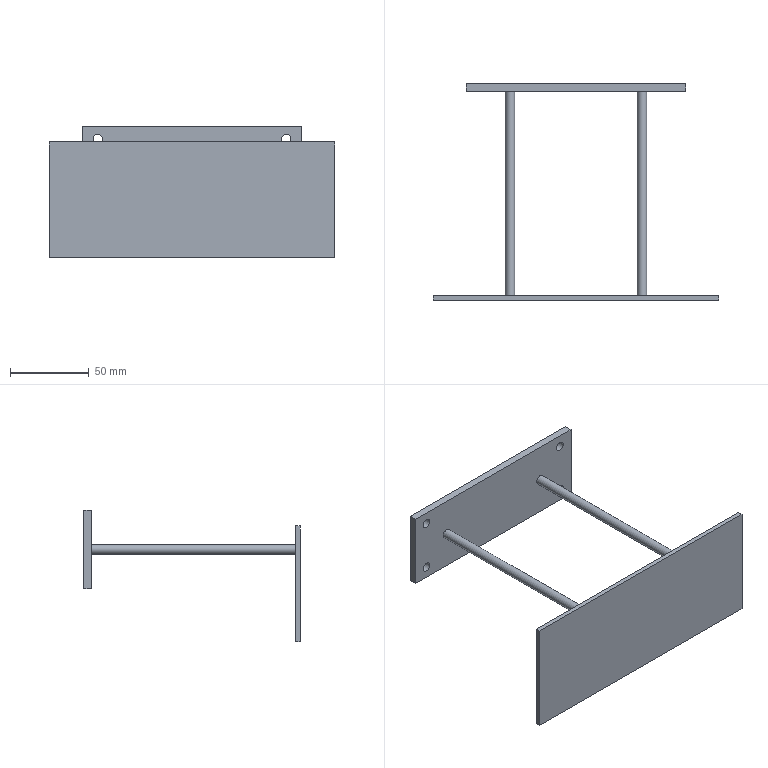Part | STEP file | zhijia | 1 solid | 18 faces | box 182 x 138 x 83.7 mm | volume 82026 mm3 | plane 12 | cylinder 6 | commonest cylinder face diameters 6 x6
STEP:
#1=CARTESIAN_POINT('',(0.,0.,0.));
#2=DIRECTION('',(0.,0.,1.));
#3=DIRECTION('',(1.,0.,0.));
#4=AXIS2_PLACEMENT_3D('',#1,#2,#3);
#5=CARTESIAN_POINT('',(-70.,-2.5,-25.));
#6=VERTEX_POINT('',#5);
#7=CARTESIAN_POINT('',(-70.,-2.5,25.));
#8=VERTEX_POINT('',#7);
#9=CARTESIAN_POINT('',(-70.,-2.5,-25.));
#10=DIRECTION('',(0.,0.,1.));
#11=VECTOR('',#10,1.);
#12=LINE('',#9,#11);
#13=CARTESIAN_POINT('',(-70.,2.5,-25.));
#14=DIRECTION('',(1.,0.,0.));
#15=DIRECTION('',(0.,0.,-1.));
#16=AXIS2_PLACEMENT_3D('',#13,#14,#15);
#17=PLANE('',#16);
#18=CARTESIAN_POINT('',(0.,-5.));
#19=DIRECTION('',(-1.,0.));
#20=VECTOR('',#19,1.);
#21=LINE('',#18,#20);
#22=(GEOMETRIC_REPRESENTATION_CONTEXT(2)PARAMETRIC_REPRESENTATION_CONTEXT()REPRESENTATION_CONTEXT('',''));
#23=DEFINITIONAL_REPRESENTATION('',(#21),#22);
#24=PCURVE('',#17,#23);
#25=CARTESIAN_POINT('',(0.,-2.5,0.));
#26=DIRECTION('',(0.,-1.,0.));
#27=DIRECTION('',(0.,0.,-1.));
#28=AXIS2_PLACEMENT_3D('',#25,#26,#27);
#29=PLANE('',#28);
#30=CARTESIAN_POINT('',(25.,-70.));
#31=DIRECTION('',(-1.,0.));
#32=VECTOR('',#31,1.);
#33=LINE('',#30,#32);
#34=(GEOMETRIC_REPRESENTATION_CONTEXT(2)PARAMETRIC_REPRESENTATION_CONTEXT()REPRESENTATION_CONTEXT('',''));
#35=DEFINITIONAL_REPRESENTATION('',(#33),#34);
#36=PCURVE('',#29,#35);
#37=SURFACE_CURVE('',#12,(#24,#36),.PCURVE_S1.);
#38=EDGE_CURVE('',#6,#8,#37,.T.);
#39=ORIENTED_EDGE('',*,*,#38,.T.);
#40=CARTESIAN_POINT('',(-70.,2.5,25.));
#41=VERTEX_POINT('',#40);
#42=CARTESIAN_POINT('',(-70.,2.5,25.));
#43=DIRECTION('',(0.,-1.,0.));
#44=VECTOR('',#43,1.);
#45=LINE('',#42,#44);
#46=CARTESIAN_POINT('',(-50.,0.));
#47=DIRECTION('',(0.,-1.));
#48=VECTOR('',#47,1.);
#49=LINE('',#46,#48);
#50=(GEOMETRIC_REPRESENTATION_CONTEXT(2)PARAMETRIC_REPRESENTATION_CONTEXT()REPRESENTATION_CONTEXT('',''));
#51=DEFINITIONAL_REPRESENTATION('',(#49),#50);
#52=PCURVE('',#17,#51);
#53=CARTESIAN_POINT('',(70.,2.5,25.));
#54=DIRECTION('',(0.,0.,-1.));
#55=DIRECTION('',(-1.,0.,0.));
#56=AXIS2_PLACEMENT_3D('',#53,#54,#55);
#57=PLANE('',#56);
#58=CARTESIAN_POINT('',(140.,0.));
#59=DIRECTION('',(0.,-1.));
#60=VECTOR('',#59,1.);
#61=LINE('',#58,#60);
#62=(GEOMETRIC_REPRESENTATION_CONTEXT(2)PARAMETRIC_REPRESENTATION_CONTEXT()REPRESENTATION_CONTEXT('',''));
#63=DEFINITIONAL_REPRESENTATION('',(#61),#62);
#64=PCURVE('',#57,#63);
#65=SURFACE_CURVE('',#45,(#52,#64),.PCURVE_S1.);
#66=EDGE_CURVE('',#41,#8,#65,.T.);
#67=ORIENTED_EDGE('',*,*,#66,.F.);
#68=CARTESIAN_POINT('',(-70.,2.5,-25.));
#69=VERTEX_POINT('',#68);
#70=CARTESIAN_POINT('',(-70.,2.5,-25.));
#71=DIRECTION('',(0.,0.,1.));
#72=VECTOR('',#71,1.);
#73=LINE('',#70,#72);
#74=CARTESIAN_POINT('',(0.,0.));
#75=DIRECTION('',(-1.,0.));
#76=VECTOR('',#75,1.);
#77=LINE('',#74,#76);
#78=(GEOMETRIC_REPRESENTATION_CONTEXT(2)PARAMETRIC_REPRESENTATION_CONTEXT()REPRESENTATION_CONTEXT('',''));
#79=DEFINITIONAL_REPRESENTATION('',(#77),#78);
#80=PCURVE('',#17,#79);
#81=CARTESIAN_POINT('',(0.,2.5,0.));
#82=DIRECTION('',(0.,-1.,0.));
#83=DIRECTION('',(0.,0.,-1.));
#84=AXIS2_PLACEMENT_3D('',#81,#82,#83);
#85=PLANE('',#84);
#86=CARTESIAN_POINT('',(25.,-70.));
#87=DIRECTION('',(-1.,0.));
#88=VECTOR('',#87,1.);
#89=LINE('',#86,#88);
#90=(GEOMETRIC_REPRESENTATION_CONTEXT(2)PARAMETRIC_REPRESENTATION_CONTEXT()REPRESENTATION_CONTEXT('',''));
#91=DEFINITIONAL_REPRESENTATION('',(#89),#90);
#92=PCURVE('',#85,#91);
#93=SURFACE_CURVE('',#73,(#80,#92),.PCURVE_S1.);
#94=EDGE_CURVE('',#69,#41,#93,.T.);
#95=ORIENTED_EDGE('',*,*,#94,.F.);
#96=CARTESIAN_POINT('',(-70.,2.5,-25.));
#97=DIRECTION('',(0.,-1.,0.));
#98=VECTOR('',#97,1.);
#99=LINE('',#96,#98);
#100=CARTESIAN_POINT('',(0.,0.));
#101=DIRECTION('',(0.,-1.));
#102=VECTOR('',#101,1.);
#103=LINE('',#100,#102);
#104=(GEOMETRIC_REPRESENTATION_CONTEXT(2)PARAMETRIC_REPRESENTATION_CONTEXT()REPRESENTATION_CONTEXT('',''));
#105=DEFINITIONAL_REPRESENTATION('',(#103),#104);
#106=PCURVE('',#17,#105);
#107=CARTESIAN_POINT('',(70.,2.5,-25.));
#108=DIRECTION('',(0.,0.,1.));
#109=DIRECTION('',(1.,0.,0.));
#110=AXIS2_PLACEMENT_3D('',#107,#108,#109);
#111=PLANE('',#110);
#112=CARTESIAN_POINT('',(-140.,0.));
#113=DIRECTION('',(0.,-1.));
#114=VECTOR('',#113,1.);
#115=LINE('',#112,#114);
#116=(GEOMETRIC_REPRESENTATION_CONTEXT(2)PARAMETRIC_REPRESENTATION_CONTEXT()REPRESENTATION_CONTEXT('',''));
#117=DEFINITIONAL_REPRESENTATION('',(#115),#116);
#118=PCURVE('',#111,#117);
#119=SURFACE_CURVE('',#99,(#106,#118),.PCURVE_S1.);
#120=EDGE_CURVE('',#69,#6,#119,.T.);
#121=ORIENTED_EDGE('',*,*,#120,.T.);
#122=EDGE_LOOP('',(#39,#67,#95,#121));
#123=FACE_BOUND('',#122,.T.);
#124=ADVANCED_FACE('',(#123),#17,.F.);
#125=CARTESIAN_POINT('',(70.,-2.5,25.));
#126=VERTEX_POINT('',#125);
#127=CARTESIAN_POINT('',(70.,-2.5,25.));
#128=DIRECTION('',(1.,0.,0.));
#129=VECTOR('',#128,1.);
#130=LINE('',#127,#129);
#131=CARTESIAN_POINT('',(0.,-5.));
#132=DIRECTION('',(-1.,0.));
#133=VECTOR('',#132,1.);
#134=LINE('',#131,#133);
#135=(GEOMETRIC_REPRESENTATION_CONTEXT(2)PARAMETRIC_REPRESENTATION_CONTEXT()REPRESENTATION_CONTEXT('',''));
#136=DEFINITIONAL_REPRESENTATION('',(#134),#135);
#137=PCURVE('',#57,#136);
#138=CARTESIAN_POINT('',(-25.,70.));
#139=DIRECTION('',(0.,1.));
#140=VECTOR('',#139,1.);
#141=LINE('',#138,#140);
#142=(GEOMETRIC_REPRESENTATION_CONTEXT(2)PARAMETRIC_REPRESENTATION_CONTEXT()REPRESENTATION_CONTEXT('',''));
#143=DEFINITIONAL_REPRESENTATION('',(#141),#142);
#144=PCURVE('',#29,#143);
#145=SURFACE_CURVE('',#130,(#137,#144),.PCURVE_S1.);
#146=EDGE_CURVE('',#8,#126,#145,.T.);
#147=ORIENTED_EDGE('',*,*,#146,.T.);
#148=CARTESIAN_POINT('',(70.,2.5,25.));
#149=VERTEX_POINT('',#148);
#150=CARTESIAN_POINT('',(70.,2.5,25.));
#151=DIRECTION('',(0.,-1.,0.));
#152=VECTOR('',#151,1.);
#153=LINE('',#150,#152);
#154=CARTESIAN_POINT('',(0.,0.));
#155=DIRECTION('',(0.,-1.));
#156=VECTOR('',#155,1.);
#157=LINE('',#154,#156);
#158=(GEOMETRIC_REPRESENTATION_CONTEXT(2)PARAMETRIC_REPRESENTATION_CONTEXT()REPRESENTATION_CONTEXT('',''));
#159=DEFINITIONAL_REPRESENTATION('',(#157),#158);
#160=PCURVE('',#57,#159);
#161=CARTESIAN_POINT('',(70.,2.5,-25.));
#162=DIRECTION('',(-1.,0.,0.));
#163=DIRECTION('',(0.,0.,1.));
#164=AXIS2_PLACEMENT_3D('',#161,#162,#163);
#165=PLANE('',#164);
#166=CARTESIAN_POINT('',(50.,0.));
#167=DIRECTION('',(0.,-1.));
#168=VECTOR('',#167,1.);
#169=LINE('',#166,#168);
#170=(GEOMETRIC_REPRESENTATION_CONTEXT(2)PARAMETRIC_REPRESENTATION_CONTEXT()REPRESENTATION_CONTEXT('',''));
#171=DEFINITIONAL_REPRESENTATION('',(#169),#170);
#172=PCURVE('',#165,#171);
#173=SURFACE_CURVE('',#153,(#160,#172),.PCURVE_S1.);
#174=EDGE_CURVE('',#149,#126,#173,.T.);
#175=ORIENTED_EDGE('',*,*,#174,.F.);
#176=CARTESIAN_POINT('',(70.,2.5,25.));
#177=DIRECTION('',(1.,0.,0.));
#178=VECTOR('',#177,1.);
#179=LINE('',#176,#178);
#180=CARTESIAN_POINT('',(0.,0.));
#181=DIRECTION('',(-1.,0.));
#182=VECTOR('',#181,1.);
#183=LINE('',#180,#182);
#184=(GEOMETRIC_REPRESENTATION_CONTEXT(2)PARAMETRIC_REPRESENTATION_CONTEXT()REPRESENTATION_CONTEXT('',''));
#185=DEFINITIONAL_REPRESENTATION('',(#183),#184);
#186=PCURVE('',#57,#185);
#187=CARTESIAN_POINT('',(-25.,70.));
#188=DIRECTION('',(0.,1.));
#189=VECTOR('',#188,1.);
#190=LINE('',#187,#189);
#191=(GEOMETRIC_REPRESENTATION_CONTEXT(2)PARAMETRIC_REPRESENTATION_CONTEXT()REPRESENTATION_CONTEXT('',''));
#192=DEFINITIONAL_REPRESENTATION('',(#190),#191);
#193=PCURVE('',#85,#192);
#194=SURFACE_CURVE('',#179,(#186,#193),.PCURVE_S1.);
#195=EDGE_CURVE('',#41,#149,#194,.T.);
#196=ORIENTED_EDGE('',*,*,#195,.F.);
#197=ORIENTED_EDGE('',*,*,#66,.T.);
#198=EDGE_LOOP('',(#147,#175,#196,#197));
#199=FACE_BOUND('',#198,.T.);
#200=ADVANCED_FACE('',(#199),#57,.F.);
#201=CARTESIAN_POINT('',(70.,-2.5,-25.));
#202=VERTEX_POINT('',#201);
#203=CARTESIAN_POINT('',(70.,-2.5,-25.));
#204=DIRECTION('',(0.,0.,-1.));
#205=VECTOR('',#204,1.);
#206=LINE('',#203,#205);
#207=CARTESIAN_POINT('',(0.,-5.));
#208=DIRECTION('',(-1.,0.));
#209=VECTOR('',#208,1.);
#210=LINE('',#207,#209);
#211=(GEOMETRIC_REPRESENTATION_CONTEXT(2)PARAMETRIC_REPRESENTATION_CONTEXT()REPRESENTATION_CONTEXT('',''));
#212=DEFINITIONAL_REPRESENTATION('',(#210),#211);
#213=PCURVE('',#165,#212);
#214=CARTESIAN_POINT('',(25.,70.));
#215=DIRECTION('',(1.,0.));
#216=VECTOR('',#215,1.);
#217=LINE('',#214,#216);
#218=(GEOMETRIC_REPRESENTATION_CONTEXT(2)PARAMETRIC_REPRESENTATION_CONTEXT()REPRESENTATION_CONTEXT('',''));
#219=DEFINITIONAL_REPRESENTATION('',(#217),#218);
#220=PCURVE('',#29,#219);
#221=SURFACE_CURVE('',#206,(#213,#220),.PCURVE_S1.);
#222=EDGE_CURVE('',#126,#202,#221,.T.);
#223=ORIENTED_EDGE('',*,*,#222,.T.);
#224=CARTESIAN_POINT('',(70.,2.5,-25.));
#225=VERTEX_POINT('',#224);
#226=CARTESIAN_POINT('',(70.,2.5,-25.));
#227=DIRECTION('',(0.,-1.,0.));
#228=VECTOR('',#227,1.);
#229=LINE('',#226,#228);
#230=CARTESIAN_POINT('',(0.,0.));
#231=DIRECTION('',(0.,-1.));
#232=VECTOR('',#231,1.);
#233=LINE('',#230,#232);
#234=(GEOMETRIC_REPRESENTATION_CONTEXT(2)PARAMETRIC_REPRESENTATION_CONTEXT()REPRESENTATION_CONTEXT('',''));
#235=DEFINITIONAL_REPRESENTATION('',(#233),#234);
#236=PCURVE('',#165,#235);
#237=CARTESIAN_POINT('',(0.,0.));
#238=DIRECTION('',(0.,-1.));
#239=VECTOR('',#238,1.);
#240=LINE('',#237,#239);
#241=(GEOMETRIC_REPRESENTATION_CONTEXT(2)PARAMETRIC_REPRESENTATION_CONTEXT()REPRESENTATION_CONTEXT('',''));
#242=DEFINITIONAL_REPRESENTATION('',(#240),#241);
#243=PCURVE('',#111,#242);
#244=SURFACE_CURVE('',#229,(#236,#243),.PCURVE_S1.);
#245=EDGE_CURVE('',#225,#202,#244,.T.);
#246=ORIENTED_EDGE('',*,*,#245,.F.);
#247=CARTESIAN_POINT('',(70.,2.5,-25.));
#248=DIRECTION('',(0.,0.,-1.));
#249=VECTOR('',#248,1.);
#250=LINE('',#247,#249);
#251=CARTESIAN_POINT('',(0.,0.));
#252=DIRECTION('',(-1.,0.));
#253=VECTOR('',#252,1.);
#254=LINE('',#251,#253);
#255=(GEOMETRIC_REPRESENTATION_CONTEXT(2)PARAMETRIC_REPRESENTATION_CONTEXT()REPRESENTATION_CONTEXT('',''));
#256=DEFINITIONAL_REPRESENTATION('',(#254),#255);
#257=PCURVE('',#165,#256);
#258=CARTESIAN_POINT('',(25.,70.));
#259=DIRECTION('',(1.,0.));
#260=VECTOR('',#259,1.);
#261=LINE('',#258,#260);
#262=(GEOMETRIC_REPRESENTATION_CONTEXT(2)PARAMETRIC_REPRESENTATION_CONTEXT()REPRESENTATION_CONTEXT('',''));
#263=DEFINITIONAL_REPRESENTATION('',(#261),#262);
#264=PCURVE('',#85,#263);
#265=SURFACE_CURVE('',#250,(#257,#264),.PCURVE_S1.);
#266=EDGE_CURVE('',#149,#225,#265,.T.);
#267=ORIENTED_EDGE('',*,*,#266,.F.);
#268=ORIENTED_EDGE('',*,*,#174,.T.);
#269=EDGE_LOOP('',(#223,#246,#267,#268));
#270=FACE_BOUND('',#269,.T.);
#271=ADVANCED_FACE('',(#270),#165,.F.);
#272=CARTESIAN_POINT('',(70.,-2.5,-25.));
#273=DIRECTION('',(-1.,0.,0.));
#274=VECTOR('',#273,1.);
#275=LINE('',#272,#274);
#276=CARTESIAN_POINT('',(0.,-5.));
#277=DIRECTION('',(-1.,0.));
#278=VECTOR('',#277,1.);
#279=LINE('',#276,#278);
#280=(GEOMETRIC_REPRESENTATION_CONTEXT(2)PARAMETRIC_REPRESENTATION_CONTEXT()REPRESENTATION_CONTEXT('',''));
#281=DEFINITIONAL_REPRESENTATION('',(#279),#280);
#282=PCURVE('',#111,#281);
#283=CARTESIAN_POINT('',(25.,70.));
#284=DIRECTION('',(0.,-1.));
#285=VECTOR('',#284,1.);
#286=LINE('',#283,#285);
#287=(GEOMETRIC_REPRESENTATION_CONTEXT(2)PARAMETRIC_REPRESENTATION_CONTEXT()REPRESENTATION_CONTEXT('',''));
#288=DEFINITIONAL_REPRESENTATION('',(#286),#287);
#289=PCURVE('',#29,#288);
#290=SURFACE_CURVE('',#275,(#282,#289),.PCURVE_S1.);
#291=EDGE_CURVE('',#202,#6,#290,.T.);
#292=ORIENTED_EDGE('',*,*,#291,.T.);
#293=ORIENTED_EDGE('',*,*,#120,.F.);
#294=CARTESIAN_POINT('',(70.,2.5,-25.));
#295=DIRECTION('',(-1.,0.,0.));
#296=VECTOR('',#295,1.);
#297=LINE('',#294,#296);
#298=CARTESIAN_POINT('',(0.,0.));
#299=DIRECTION('',(-1.,0.));
#300=VECTOR('',#299,1.);
#301=LINE('',#298,#300);
#302=(GEOMETRIC_REPRESENTATION_CONTEXT(2)PARAMETRIC_REPRESENTATION_CONTEXT()REPRESENTATION_CONTEXT('',''));
#303=DEFINITIONAL_REPRESENTATION('',(#301),#302);
#304=PCURVE('',#111,#303);
#305=CARTESIAN_POINT('',(25.,70.));
#306=DIRECTION('',(0.,-1.));
#307=VECTOR('',#306,1.);
#308=LINE('',#305,#307);
#309=(GEOMETRIC_REPRESENTATION_CONTEXT(2)PARAMETRIC_REPRESENTATION_CONTEXT()REPRESENTATION_CONTEXT('',''));
#310=DEFINITIONAL_REPRESENTATION('',(#308),#309);
#311=PCURVE('',#85,#310);
#312=SURFACE_CURVE('',#297,(#304,#311),.PCURVE_S1.);
#313=EDGE_CURVE('',#225,#69,#312,.T.);
#314=ORIENTED_EDGE('',*,*,#313,.F.);
#315=ORIENTED_EDGE('',*,*,#245,.T.);
#316=EDGE_LOOP('',(#292,#293,#314,#315));
#317=FACE_BOUND('',#316,.T.);
#318=ADVANCED_FACE('',(#317),#111,.F.);
#319=CARTESIAN_POINT('',(-60.,2.5,20.));
#320=VERTEX_POINT('',#319);
#321=CARTESIAN_POINT('',(-60.,2.5,17.));
#322=DIRECTION('',(0.,1.,0.));
#323=DIRECTION('',(0.,0.,1.));
#324=AXIS2_PLACEMENT_3D('',#321,#322,#323);
#325=CIRCLE('',#324,3.);
#326=CARTESIAN_POINT('',(-20.,-60.));
#327=CARTESIAN_POINT('',(-20.,-54.804));
#328=CARTESIAN_POINT('',(-15.5,-57.402));
#329=CARTESIAN_POINT('',(-11.,-60.));
#330=CARTESIAN_POINT('',(-15.5,-62.598));
#331=CARTESIAN_POINT('',(-20.,-65.196));
#332=CARTESIAN_POINT('',(-20.,-60.));
#333=(BOUNDED_CURVE()B_SPLINE_CURVE(2,(#326,#327,#328,#329,#330,#331,#332),.UNSPECIFIED.,.T.,.F.)B_SPLINE_CURVE_WITH_KNOTS((1,2,2,2,2,1),(-2.094,0.,2.094,4.189,6.283,8.378),.UNSPECIFIED.)CURVE()GEOMETRIC_REPRESENTATION_ITEM()RATIONAL_B_SPLINE_CURVE((1.,0.5,1.,0.5,1.,0.5,1.))REPRESENTATION_ITEM(''));
#334=(GEOMETRIC_REPRESENTATION_CONTEXT(2)PARAMETRIC_REPRESENTATION_CONTEXT()REPRESENTATION_CONTEXT('',''));
#335=DEFINITIONAL_REPRESENTATION('',(#333),#334);
#336=PCURVE('',#85,#335);
#337=CARTESIAN_POINT('',(-60.,-2.5,17.));
#338=DIRECTION('',(0.,1.,0.));
#339=DIRECTION('',(0.,0.,1.));
#340=AXIS2_PLACEMENT_3D('',#337,#338,#339);
#341=CYLINDRICAL_SURFACE('',#340,3.);
#342=CARTESIAN_POINT('',(0.,5.));
#343=DIRECTION('',(1.,0.));
#344=VECTOR('',#343,1.);
#345=LINE('',#342,#344);
#346=(GEOMETRIC_REPRESENTATION_CONTEXT(2)PARAMETRIC_REPRESENTATION_CONTEXT()REPRESENTATION_CONTEXT('',''));
#347=DEFINITIONAL_REPRESENTATION('',(#345),#346);
#348=PCURVE('',#341,#347);
#349=SURFACE_CURVE('',#325,(#336,#348),.PCURVE_S1.);
#350=EDGE_CURVE('',#320,#320,#349,.T.);
#351=ORIENTED_EDGE('',*,*,#350,.F.);
#352=EDGE_LOOP('',(#351));
#353=FACE_BOUND('',#352,.T.);
#354=CARTESIAN_POINT('',(60.,2.5,14.));
#355=VERTEX_POINT('',#354);
#356=CARTESIAN_POINT('',(60.,2.5,17.));
#357=DIRECTION('',(0.,1.,0.));
#358=DIRECTION('',(0.,0.,-1.));
#359=AXIS2_PLACEMENT_3D('',#356,#357,#358);
#360=CIRCLE('',#359,3.);
#361=CARTESIAN_POINT('',(-14.,60.));
#362=CARTESIAN_POINT('',(-14.,54.804));
#363=CARTESIAN_POINT('',(-18.5,57.402));
#364=CARTESIAN_POINT('',(-23.,60.));
#365=CARTESIAN_POINT('',(-18.5,62.598));
#366=CARTESIAN_POINT('',(-14.,65.196));
#367=CARTESIAN_POINT('',(-14.,60.));
#368=(BOUNDED_CURVE()B_SPLINE_CURVE(2,(#361,#362,#363,#364,#365,#366,#367),.UNSPECIFIED.,.T.,.F.)B_SPLINE_CURVE_WITH_KNOTS((1,2,2,2,2,1),(-2.094,0.,2.094,4.189,6.283,8.378),.UNSPECIFIED.)CURVE()GEOMETRIC_REPRESENTATION_ITEM()RATIONAL_B_SPLINE_CURVE((1.,0.5,1.,0.5,1.,0.5,1.))REPRESENTATION_ITEM(''));
#369=(GEOMETRIC_REPRESENTATION_CONTEXT(2)PARAMETRIC_REPRESENTATION_CONTEXT()REPRESENTATION_CONTEXT('',''));
#370=DEFINITIONAL_REPRESENTATION('',(#368),#369);
#371=PCURVE('',#85,#370);
#372=CARTESIAN_POINT('',(60.,-2.5,17.));
#373=DIRECTION('',(0.,1.,0.));
#374=DIRECTION('',(0.,0.,1.));
#375=AXIS2_PLACEMENT_3D('',#372,#373,#374);
#376=CYLINDRICAL_SURFACE('',#375,3.);
#377=CARTESIAN_POINT('',(3.142,5.));
#378=DIRECTION('',(1.,0.));
#379=VECTOR('',#378,1.);
#380=LINE('',#377,#379);
#381=(GEOMETRIC_REPRESENTATION_CONTEXT(2)PARAMETRIC_REPRESENTATION_CONTEXT()REPRESENTATION_CONTEXT('',''));
#382=DEFINITIONAL_REPRESENTATION('',(#380),#381);
#383=PCURVE('',#376,#382);
#384=SURFACE_CURVE('',#360,(#371,#383),.PCURVE_S1.);
#385=EDGE_CURVE('',#355,#355,#384,.T.);
#386=ORIENTED_EDGE('',*,*,#385,.F.);
#387=EDGE_LOOP('',(#386));
#388=FACE_BOUND('',#387,.T.);
#389=CARTESIAN_POINT('',(60.,2.5,-20.));
#390=VERTEX_POINT('',#389);
#391=CARTESIAN_POINT('',(60.,2.5,-17.));
#392=DIRECTION('',(0.,1.,0.));
#393=DIRECTION('',(0.,0.,-1.));
#394=AXIS2_PLACEMENT_3D('',#391,#392,#393);
#395=CIRCLE('',#394,3.);
#396=CARTESIAN_POINT('',(20.,60.));
#397=CARTESIAN_POINT('',(20.,54.804));
#398=CARTESIAN_POINT('',(15.5,57.402));
#399=CARTESIAN_POINT('',(11.,60.));
#400=CARTESIAN_POINT('',(15.5,62.598));
#401=CARTESIAN_POINT('',(20.,65.196));
#402=CARTESIAN_POINT('',(20.,60.));
#403=(BOUNDED_CURVE()B_SPLINE_CURVE(2,(#396,#397,#398,#399,#400,#401,#402),.UNSPECIFIED.,.T.,.F.)B_SPLINE_CURVE_WITH_KNOTS((1,2,2,2,2,1),(-2.094,0.,2.094,4.189,6.283,8.378),.UNSPECIFIED.)CURVE()GEOMETRIC_REPRESENTATION_ITEM()RATIONAL_B_SPLINE_CURVE((1.,0.5,1.,0.5,1.,0.5,1.))REPRESENTATION_ITEM(''));
#404=(GEOMETRIC_REPRESENTATION_CONTEXT(2)PARAMETRIC_REPRESENTATION_CONTEXT()REPRESENTATION_CONTEXT('',''));
#405=DEFINITIONAL_REPRESENTATION('',(#403),#404);
#406=PCURVE('',#85,#405);
#407=CARTESIAN_POINT('',(60.,-2.5,-17.));
#408=DIRECTION('',(0.,1.,0.));
#409=DIRECTION('',(0.,0.,1.));
#410=AXIS2_PLACEMENT_3D('',#407,#408,#409);
#411=CYLINDRICAL_SURFACE('',#410,3.);
#412=CARTESIAN_POINT('',(3.142,5.));
#413=DIRECTION('',(1.,0.));
#414=VECTOR('',#413,1.);
#415=LINE('',#412,#414);
#416=(GEOMETRIC_REPRESENTATION_CONTEXT(2)PARAMETRIC_REPRESENTATION_CONTEXT()REPRESENTATION_CONTEXT('',''));
#417=DEFINITIONAL_REPRESENTATION('',(#415),#416);
#418=PCURVE('',#411,#417);
#419=SURFACE_CURVE('',#395,(#406,#418),.PCURVE_S1.);
#420=EDGE_CURVE('',#390,#390,#419,.T.);
#421=ORIENTED_EDGE('',*,*,#420,.F.);
#422=EDGE_LOOP('',(#421));
#423=FACE_BOUND('',#422,.T.);
#424=CARTESIAN_POINT('',(-60.,2.5,-14.));
#425=VERTEX_POINT('',#424);
#426=CARTESIAN_POINT('',(-60.,2.5,-17.));
#427=DIRECTION('',(0.,1.,0.));
#428=DIRECTION('',(0.,0.,1.));
#429=AXIS2_PLACEMENT_3D('',#426,#427,#428);
#430=CIRCLE('',#429,3.);
#431=CARTESIAN_POINT('',(14.,-60.));
#432=CARTESIAN_POINT('',(14.,-54.804));
#433=CARTESIAN_POINT('',(18.5,-57.402));
#434=CARTESIAN_POINT('',(23.,-60.));
#435=CARTESIAN_POINT('',(18.5,-62.598));
#436=CARTESIAN_POINT('',(14.,-65.196));
#437=CARTESIAN_POINT('',(14.,-60.));
#438=(BOUNDED_CURVE()B_SPLINE_CURVE(2,(#431,#432,#433,#434,#435,#436,#437),.UNSPECIFIED.,.T.,.F.)B_SPLINE_CURVE_WITH_KNOTS((1,2,2,2,2,1),(-2.094,0.,2.094,4.189,6.283,8.378),.UNSPECIFIED.)CURVE()GEOMETRIC_REPRESENTATION_ITEM()RATIONAL_B_SPLINE_CURVE((1.,0.5,1.,0.5,1.,0.5,1.))REPRESENTATION_ITEM(''));
#439=(GEOMETRIC_REPRESENTATION_CONTEXT(2)PARAMETRIC_REPRESENTATION_CONTEXT()REPRESENTATION_CONTEXT('',''));
#440=DEFINITIONAL_REPRESENTATION('',(#438),#439);
#441=PCURVE('',#85,#440);
#442=CARTESIAN_POINT('',(-60.,-2.5,-17.));
#443=DIRECTION('',(0.,1.,0.));
#444=DIRECTION('',(0.,0.,1.));
#445=AXIS2_PLACEMENT_3D('',#442,#443,#444);
#446=CYLINDRICAL_SURFACE('',#445,3.);
#447=CARTESIAN_POINT('',(0.,5.));
#448=DIRECTION('',(1.,0.));
#449=VECTOR('',#448,1.);
#450=LINE('',#447,#449);
#451=(GEOMETRIC_REPRESENTATION_CONTEXT(2)PARAMETRIC_REPRESENTATION_CONTEXT()REPRESENTATION_CONTEXT('',''));
#452=DEFINITIONAL_REPRESENTATION('',(#450),#451);
#453=PCURVE('',#446,#452);
#454=SURFACE_CURVE('',#430,(#441,#453),.PCURVE_S1.);
#455=EDGE_CURVE('',#425,#425,#454,.T.);
#456=ORIENTED_EDGE('',*,*,#455,.F.);
#457=EDGE_LOOP('',(#456));
#458=FACE_BOUND('',#457,.T.);
#459=ORIENTED_EDGE('',*,*,#94,.T.);
#460=ORIENTED_EDGE('',*,*,#195,.T.);
#461=ORIENTED_EDGE('',*,*,#266,.T.);
#462=ORIENTED_EDGE('',*,*,#313,.T.);
#463=EDGE_LOOP('',(#459,#460,#461,#462));
#464=FACE_BOUND('',#463,.T.);
#465=ADVANCED_FACE('',(#353,#388,#423,#458,#464),#85,.F.);
#466=CARTESIAN_POINT('',(42.,-2.5,3.));
#467=VERTEX_POINT('',#466);
#468=CARTESIAN_POINT('',(42.,-2.5,0.));
#469=DIRECTION('',(0.,-1.,0.));
#470=DIRECTION('',(0.,0.,1.));
#471=AXIS2_PLACEMENT_3D('',#468,#469,#470);
#472=CIRCLE('',#471,3.);
#473=CARTESIAN_POINT('',(0.,42.));
#474=DIRECTION('',(-1.,0.));
#475=AXIS2_PLACEMENT_2D('',#473,#474);
#476=CIRCLE('',#475,3.);
#477=(GEOMETRIC_REPRESENTATION_CONTEXT(2)PARAMETRIC_REPRESENTATION_CONTEXT()REPRESENTATION_CONTEXT('',''));
#478=DEFINITIONAL_REPRESENTATION('',(#476),#477);
#479=PCURVE('',#29,#478);
#480=CARTESIAN_POINT('',(42.,-132.5,0.));
#481=DIRECTION('',(0.,1.,0.));
#482=DIRECTION('',(0.,0.,1.));
#483=AXIS2_PLACEMENT_3D('',#480,#481,#482);
#484=CYLINDRICAL_SURFACE('',#483,3.);
#485=CARTESIAN_POINT('',(6.283,130.));
#486=DIRECTION('',(-1.,0.));
#487=VECTOR('',#486,1.);
#488=LINE('',#485,#487);
#489=(GEOMETRIC_REPRESENTATION_CONTEXT(2)PARAMETRIC_REPRESENTATION_CONTEXT()REPRESENTATION_CONTEXT('',''));
#490=DEFINITIONAL_REPRESENTATION('',(#488),#489);
#491=PCURVE('',#484,#490);
#492=SURFACE_CURVE('',#472,(#479,#491),.PCURVE_S1.);
#493=EDGE_CURVE('',#467,#467,#492,.T.);
#494=ORIENTED_EDGE('',*,*,#493,.F.);
#495=EDGE_LOOP('',(#494));
#496=FACE_BOUND('',#495,.T.);
#497=CARTESIAN_POINT('',(-42.,-2.5,-3.));
#498=VERTEX_POINT('',#497);
#499=CARTESIAN_POINT('',(-42.,-2.5,0.));
#500=DIRECTION('',(0.,-1.,0.));
#501=DIRECTION('',(0.,0.,-1.));
#502=AXIS2_PLACEMENT_3D('',#499,#500,#501);
#503=CIRCLE('',#502,3.);
#504=CARTESIAN_POINT('',(0.,-42.));
#505=DIRECTION('',(1.,0.));
#506=AXIS2_PLACEMENT_2D('',#504,#505);
#507=CIRCLE('',#506,3.);
#508=(GEOMETRIC_REPRESENTATION_CONTEXT(2)PARAMETRIC_REPRESENTATION_CONTEXT()REPRESENTATION_CONTEXT('',''));
#509=DEFINITIONAL_REPRESENTATION('',(#507),#508);
#510=PCURVE('',#29,#509);
#511=CARTESIAN_POINT('',(-42.,-132.5,0.));
#512=DIRECTION('',(0.,1.,0.));
#513=DIRECTION('',(0.,0.,1.));
#514=AXIS2_PLACEMENT_3D('',#511,#512,#513);
#515=CYLINDRICAL_SURFACE('',#514,3.);
#516=CARTESIAN_POINT('',(9.425,130.));
#517=DIRECTION('',(-1.,0.));
#518=VECTOR('',#517,1.);
#519=LINE('',#516,#518);
#520=(GEOMETRIC_REPRESENTATION_CONTEXT(2)PARAMETRIC_REPRESENTATION_CONTEXT()REPRESENTATION_CONTEXT('',''));
#521=DEFINITIONAL_REPRESENTATION('',(#519),#520);
#522=PCURVE('',#515,#521);
#523=SURFACE_CURVE('',#503,(#510,#522),.PCURVE_S1.);
#524=EDGE_CURVE('',#498,#498,#523,.T.);
#525=ORIENTED_EDGE('',*,*,#524,.F.);
#526=EDGE_LOOP('',(#525));
#527=FACE_BOUND('',#526,.T.);
#528=CARTESIAN_POINT('',(-60.,-2.5,20.));
#529=VERTEX_POINT('',#528);
#530=CARTESIAN_POINT('',(-60.,-2.5,17.));
#531=DIRECTION('',(0.,1.,0.));
#532=DIRECTION('',(0.,0.,1.));
#533=AXIS2_PLACEMENT_3D('',#530,#531,#532);
#534=CIRCLE('',#533,3.);
#535=CARTESIAN_POINT('',(-20.,-60.));
#536=CARTESIAN_POINT('',(-20.,-54.804));
#537=CARTESIAN_POINT('',(-15.5,-57.402));
#538=CARTESIAN_POINT('',(-11.,-60.));
#539=CARTESIAN_POINT('',(-15.5,-62.598));
#540=CARTESIAN_POINT('',(-20.,-65.196));
#541=CARTESIAN_POINT('',(-20.,-60.));
#542=(BOUNDED_CURVE()B_SPLINE_CURVE(2,(#535,#536,#537,#538,#539,#540,#541),.UNSPECIFIED.,.T.,.F.)B_SPLINE_CURVE_WITH_KNOTS((1,2,2,2,2,1),(-2.094,0.,2.094,4.189,6.283,8.378),.UNSPECIFIED.)CURVE()GEOMETRIC_REPRESENTATION_ITEM()RATIONAL_B_SPLINE_CURVE((1.,0.5,1.,0.5,1.,0.5,1.))REPRESENTATION_ITEM(''));
#543=(GEOMETRIC_REPRESENTATION_CONTEXT(2)PARAMETRIC_REPRESENTATION_CONTEXT()REPRESENTATION_CONTEXT('',''));
#544=DEFINITIONAL_REPRESENTATION('',(#542),#543);
#545=PCURVE('',#29,#544);
#546=CARTESIAN_POINT('',(0.,0.));
#547=DIRECTION('',(1.,0.));
#548=VECTOR('',#547,1.);
#549=LINE('',#546,#548);
#550=(GEOMETRIC_REPRESENTATION_CONTEXT(2)PARAMETRIC_REPRESENTATION_CONTEXT()REPRESENTATION_CONTEXT('',''));
#551=DEFINITIONAL_REPRESENTATION('',(#549),#550);
#552=PCURVE('',#341,#551);
#553=SURFACE_CURVE('',#534,(#545,#552),.PCURVE_S1.);
#554=EDGE_CURVE('',#529,#529,#553,.T.);
#555=ORIENTED_EDGE('',*,*,#554,.T.);
#556=EDGE_LOOP('',(#555));
#557=FACE_BOUND('',#556,.T.);
#558=CARTESIAN_POINT('',(60.,-2.5,14.));
#559=VERTEX_POINT('',#558);
#560=CARTESIAN_POINT('',(60.,-2.5,17.));
#561=DIRECTION('',(0.,1.,0.));
#562=DIRECTION('',(0.,0.,-1.));
#563=AXIS2_PLACEMENT_3D('',#560,#561,#562);
#564=CIRCLE('',#563,3.);
#565=CARTESIAN_POINT('',(-14.,60.));
#566=CARTESIAN_POINT('',(-14.,54.804));
#567=CARTESIAN_POINT('',(-18.5,57.402));
#568=CARTESIAN_POINT('',(-23.,60.));
#569=CARTESIAN_POINT('',(-18.5,62.598));
#570=CARTESIAN_POINT('',(-14.,65.196));
#571=CARTESIAN_POINT('',(-14.,60.));
#572=(BOUNDED_CURVE()B_SPLINE_CURVE(2,(#565,#566,#567,#568,#569,#570,#571),.UNSPECIFIED.,.T.,.F.)B_SPLINE_CURVE_WITH_KNOTS((1,2,2,2,2,1),(-2.094,0.,2.094,4.189,6.283,8.378),.UNSPECIFIED.)CURVE()GEOMETRIC_REPRESENTATION_ITEM()RATIONAL_B_SPLINE_CURVE((1.,0.5,1.,0.5,1.,0.5,1.))REPRESENTATION_ITEM(''));
#573=(GEOMETRIC_REPRESENTATION_CONTEXT(2)PARAMETRIC_REPRESENTATION_CONTEXT()REPRESENTATION_CONTEXT('',''));
#574=DEFINITIONAL_REPRESENTATION('',(#572),#573);
#575=PCURVE('',#29,#574);
#576=CARTESIAN_POINT('',(3.142,0.));
#577=DIRECTION('',(1.,0.));
#578=VECTOR('',#577,1.);
#579=LINE('',#576,#578);
#580=(GEOMETRIC_REPRESENTATION_CONTEXT(2)PARAMETRIC_REPRESENTATION_CONTEXT()REPRESENTATION_CONTEXT('',''));
#581=DEFINITIONAL_REPRESENTATION('',(#579),#580);
#582=PCURVE('',#376,#581);
#583=SURFACE_CURVE('',#564,(#575,#582),.PCURVE_S1.);
#584=EDGE_CURVE('',#559,#559,#583,.T.);
#585=ORIENTED_EDGE('',*,*,#584,.T.);
#586=EDGE_LOOP('',(#585));
#587=FACE_BOUND('',#586,.T.);
#588=CARTESIAN_POINT('',(60.,-2.5,-20.));
#589=VERTEX_POINT('',#588);
#590=CARTESIAN_POINT('',(60.,-2.5,-17.));
#591=DIRECTION('',(0.,1.,0.));
#592=DIRECTION('',(0.,0.,-1.));
#593=AXIS2_PLACEMENT_3D('',#590,#591,#592);
#594=CIRCLE('',#593,3.);
#595=CARTESIAN_POINT('',(20.,60.));
#596=CARTESIAN_POINT('',(20.,54.804));
#597=CARTESIAN_POINT('',(15.5,57.402));
#598=CARTESIAN_POINT('',(11.,60.));
#599=CARTESIAN_POINT('',(15.5,62.598));
#600=CARTESIAN_POINT('',(20.,65.196));
#601=CARTESIAN_POINT('',(20.,60.));
#602=(BOUNDED_CURVE()B_SPLINE_CURVE(2,(#595,#596,#597,#598,#599,#600,#601),.UNSPECIFIED.,.T.,.F.)B_SPLINE_CURVE_WITH_KNOTS((1,2,2,2,2,1),(-2.094,0.,2.094,4.189,6.283,8.378),.UNSPECIFIED.)CURVE()GEOMETRIC_REPRESENTATION_ITEM()RATIONAL_B_SPLINE_CURVE((1.,0.5,1.,0.5,1.,0.5,1.))REPRESENTATION_ITEM(''));
#603=(GEOMETRIC_REPRESENTATION_CONTEXT(2)PARAMETRIC_REPRESENTATION_CONTEXT()REPRESENTATION_CONTEXT('',''));
#604=DEFINITIONAL_REPRESENTATION('',(#602),#603);
#605=PCURVE('',#29,#604);
#606=CARTESIAN_POINT('',(3.142,0.));
#607=DIRECTION('',(1.,0.));
#608=VECTOR('',#607,1.);
#609=LINE('',#606,#608);
#610=(GEOMETRIC_REPRESENTATION_CONTEXT(2)PARAMETRIC_REPRESENTATION_CONTEXT()REPRESENTATION_CONTEXT('',''));
#611=DEFINITIONAL_REPRESENTATION('',(#609),#610);
#612=PCURVE('',#411,#611);
#613=SURFACE_CURVE('',#594,(#605,#612),.PCURVE_S1.);
#614=EDGE_CURVE('',#589,#589,#613,.T.);
#615=ORIENTED_EDGE('',*,*,#614,.T.);
#616=EDGE_LOOP('',(#615));
#617=FACE_BOUND('',#616,.T.);
#618=CARTESIAN_POINT('',(-60.,-2.5,-14.));
#619=VERTEX_POINT('',#618);
#620=CARTESIAN_POINT('',(-60.,-2.5,-17.));
#621=DIRECTION('',(0.,1.,0.));
#622=DIRECTION('',(0.,0.,1.));
#623=AXIS2_PLACEMENT_3D('',#620,#621,#622);
#624=CIRCLE('',#623,3.);
#625=CARTESIAN_POINT('',(14.,-60.));
#626=CARTESIAN_POINT('',(14.,-54.804));
#627=CARTESIAN_POINT('',(18.5,-57.402));
#628=CARTESIAN_POINT('',(23.,-60.));
#629=CARTESIAN_POINT('',(18.5,-62.598));
#630=CARTESIAN_POINT('',(14.,-65.196));
#631=CARTESIAN_POINT('',(14.,-60.));
#632=(BOUNDED_CURVE()B_SPLINE_CURVE(2,(#625,#626,#627,#628,#629,#630,#631),.UNSPECIFIED.,.T.,.F.)B_SPLINE_CURVE_WITH_KNOTS((1,2,2,2,2,1),(-2.094,0.,2.094,4.189,6.283,8.378),.UNSPECIFIED.)CURVE()GEOMETRIC_REPRESENTATION_ITEM()RATIONAL_B_SPLINE_CURVE((1.,0.5,1.,0.5,1.,0.5,1.))REPRESENTATION_ITEM(''));
#633=(GEOMETRIC_REPRESENTATION_CONTEXT(2)PARAMETRIC_REPRESENTATION_CONTEXT()REPRESENTATION_CONTEXT('',''));
#634=DEFINITIONAL_REPRESENTATION('',(#632),#633);
#635=PCURVE('',#29,#634);
#636=CARTESIAN_POINT('',(0.,0.));
#637=DIRECTION('',(1.,0.));
#638=VECTOR('',#637,1.);
#639=LINE('',#636,#638);
#640=(GEOMETRIC_REPRESENTATION_CONTEXT(2)PARAMETRIC_REPRESENTATION_CONTEXT()REPRESENTATION_CONTEXT('',''));
#641=DEFINITIONAL_REPRESENTATION('',(#639),#640);
#642=PCURVE('',#446,#641);
#643=SURFACE_CURVE('',#624,(#635,#642),.PCURVE_S1.);
#644=EDGE_CURVE('',#619,#619,#643,.T.);
#645=ORIENTED_EDGE('',*,*,#644,.T.);
#646=EDGE_LOOP('',(#645));
#647=FACE_BOUND('',#646,.T.);
#648=ORIENTED_EDGE('',*,*,#38,.F.);
#649=ORIENTED_EDGE('',*,*,#291,.F.);
#650=ORIENTED_EDGE('',*,*,#222,.F.);
#651=ORIENTED_EDGE('',*,*,#146,.F.);
#652=EDGE_LOOP('',(#648,#649,#650,#651));
#653=FACE_BOUND('',#652,.T.);
#654=ADVANCED_FACE('',(#496,#527,#557,#587,#617,#647,#653),#29,.T.);
#655=ORIENTED_EDGE('',*,*,#644,.T.);
#656=CARTESIAN_POINT('',(-60.,-2.5,-14.));
#657=CARTESIAN_POINT('',(-60.,2.5,-14.));
#658=B_SPLINE_CURVE_WITH_KNOTS('',1,(#656,#657),.UNSPECIFIED.,.F.,.F.,(2,2),(0.,5.),.PIECEWISE_BEZIER_KNOTS.);
#659=CARTESIAN_POINT('',(6.283,0.));
#660=DIRECTION('',(0.,1.));
#661=VECTOR('',#660,1.);
#662=LINE('',#659,#661);
#663=(GEOMETRIC_REPRESENTATION_CONTEXT(2)PARAMETRIC_REPRESENTATION_CONTEXT()REPRESENTATION_CONTEXT('',''));
#664=DEFINITIONAL_REPRESENTATION('',(#662),#663);
#665=PCURVE('',#446,#664);
#666=CARTESIAN_POINT('',(0.,0.));
#667=DIRECTION('',(0.,1.));
#668=VECTOR('',#667,1.);
#669=LINE('',#666,#668);
#670=(GEOMETRIC_REPRESENTATION_CONTEXT(2)PARAMETRIC_REPRESENTATION_CONTEXT()REPRESENTATION_CONTEXT('',''));
#671=DEFINITIONAL_REPRESENTATION('',(#669),#670);
#672=PCURVE('',#446,#671);
#673=SEAM_CURVE('',#658,(#665,#672),.PCURVE_S1.);
#674=EDGE_CURVE('',#619,#425,#673,.T.);
#675=ORIENTED_EDGE('',*,*,#674,.T.);
#676=ORIENTED_EDGE('',*,*,#455,.F.);
#677=ORIENTED_EDGE('',*,*,#674,.F.);
#678=EDGE_LOOP('',(#655,#675,#676,#677));
#679=FACE_BOUND('',#678,.F.);
#680=ADVANCED_FACE('',(#679),#446,.F.);
#681=ORIENTED_EDGE('',*,*,#614,.T.);
#682=CARTESIAN_POINT('',(60.,-2.5,-20.));
#683=CARTESIAN_POINT('',(60.,2.5,-20.));
#684=B_SPLINE_CURVE_WITH_KNOTS('',1,(#682,#683),.UNSPECIFIED.,.F.,.F.,(2,2),(0.,5.),.PIECEWISE_BEZIER_KNOTS.);
#685=CARTESIAN_POINT('',(9.425,0.));
#686=DIRECTION('',(0.,1.));
#687=VECTOR('',#686,1.);
#688=LINE('',#685,#687);
#689=(GEOMETRIC_REPRESENTATION_CONTEXT(2)PARAMETRIC_REPRESENTATION_CONTEXT()REPRESENTATION_CONTEXT('',''));
#690=DEFINITIONAL_REPRESENTATION('',(#688),#689);
#691=PCURVE('',#411,#690);
#692=CARTESIAN_POINT('',(3.142,0.));
#693=DIRECTION('',(0.,1.));
#694=VECTOR('',#693,1.);
#695=LINE('',#692,#694);
#696=(GEOMETRIC_REPRESENTATION_CONTEXT(2)PARAMETRIC_REPRESENTATION_CONTEXT()REPRESENTATION_CONTEXT('',''));
#697=DEFINITIONAL_REPRESENTATION('',(#695),#696);
#698=PCURVE('',#411,#697);
#699=SEAM_CURVE('',#684,(#691,#698),.PCURVE_S1.);
#700=EDGE_CURVE('',#589,#390,#699,.T.);
#701=ORIENTED_EDGE('',*,*,#700,.T.);
#702=ORIENTED_EDGE('',*,*,#420,.F.);
#703=ORIENTED_EDGE('',*,*,#700,.F.);
#704=EDGE_LOOP('',(#681,#701,#702,#703));
#705=FACE_BOUND('',#704,.F.);
#706=ADVANCED_FACE('',(#705),#411,.F.);
#707=ORIENTED_EDGE('',*,*,#584,.T.);
#708=CARTESIAN_POINT('',(60.,-2.5,14.));
#709=CARTESIAN_POINT('',(60.,2.5,14.));
#710=B_SPLINE_CURVE_WITH_KNOTS('',1,(#708,#709),.UNSPECIFIED.,.F.,.F.,(2,2),(0.,5.),.PIECEWISE_BEZIER_KNOTS.);
#711=CARTESIAN_POINT('',(9.425,0.));
#712=DIRECTION('',(0.,1.));
#713=VECTOR('',#712,1.);
#714=LINE('',#711,#713);
#715=(GEOMETRIC_REPRESENTATION_CONTEXT(2)PARAMETRIC_REPRESENTATION_CONTEXT()REPRESENTATION_CONTEXT('',''));
#716=DEFINITIONAL_REPRESENTATION('',(#714),#715);
#717=PCURVE('',#376,#716);
#718=CARTESIAN_POINT('',(3.142,0.));
#719=DIRECTION('',(0.,1.));
#720=VECTOR('',#719,1.);
#721=LINE('',#718,#720);
#722=(GEOMETRIC_REPRESENTATION_CONTEXT(2)PARAMETRIC_REPRESENTATION_CONTEXT()REPRESENTATION_CONTEXT('',''));
#723=DEFINITIONAL_REPRESENTATION('',(#721),#722);
#724=PCURVE('',#376,#723);
#725=SEAM_CURVE('',#710,(#717,#724),.PCURVE_S1.);
#726=EDGE_CURVE('',#559,#355,#725,.T.);
#727=ORIENTED_EDGE('',*,*,#726,.T.);
#728=ORIENTED_EDGE('',*,*,#385,.F.);
#729=ORIENTED_EDGE('',*,*,#726,.F.);
#730=EDGE_LOOP('',(#707,#727,#728,#729));
#731=FACE_BOUND('',#730,.F.);
#732=ADVANCED_FACE('',(#731),#376,.F.);
#733=ORIENTED_EDGE('',*,*,#554,.T.);
#734=CARTESIAN_POINT('',(-60.,-2.5,20.));
#735=CARTESIAN_POINT('',(-60.,2.5,20.));
#736=B_SPLINE_CURVE_WITH_KNOTS('',1,(#734,#735),.UNSPECIFIED.,.F.,.F.,(2,2),(0.,5.),.PIECEWISE_BEZIER_KNOTS.);
#737=CARTESIAN_POINT('',(6.283,0.));
#738=DIRECTION('',(0.,1.));
#739=VECTOR('',#738,1.);
#740=LINE('',#737,#739);
#741=(GEOMETRIC_REPRESENTATION_CONTEXT(2)PARAMETRIC_REPRESENTATION_CONTEXT()REPRESENTATION_CONTEXT('',''));
#742=DEFINITIONAL_REPRESENTATION('',(#740),#741);
#743=PCURVE('',#341,#742);
#744=CARTESIAN_POINT('',(0.,0.));
#745=DIRECTION('',(0.,1.));
#746=VECTOR('',#745,1.);
#747=LINE('',#744,#746);
#748=(GEOMETRIC_REPRESENTATION_CONTEXT(2)PARAMETRIC_REPRESENTATION_CONTEXT()REPRESENTATION_CONTEXT('',''));
#749=DEFINITIONAL_REPRESENTATION('',(#747),#748);
#750=PCURVE('',#341,#749);
#751=SEAM_CURVE('',#736,(#743,#750),.PCURVE_S1.);
#752=EDGE_CURVE('',#529,#320,#751,.T.);
#753=ORIENTED_EDGE('',*,*,#752,.T.);
#754=ORIENTED_EDGE('',*,*,#350,.F.);
#755=ORIENTED_EDGE('',*,*,#752,.F.);
#756=EDGE_LOOP('',(#733,#753,#754,#755));
#757=FACE_BOUND('',#756,.F.);
#758=ADVANCED_FACE('',(#757),#341,.F.);
#759=CARTESIAN_POINT('',(-42.,-132.5,-3.));
#760=VERTEX_POINT('',#759);
#761=CARTESIAN_POINT('',(-42.,-132.5,0.));
#762=DIRECTION('',(0.,-1.,0.));
#763=DIRECTION('',(0.,0.,-1.));
#764=AXIS2_PLACEMENT_3D('',#761,#762,#763);
#765=CIRCLE('',#764,3.);
#766=CARTESIAN_POINT('',(9.425,0.));
#767=DIRECTION('',(-1.,0.));
#768=VECTOR('',#767,1.);
#769=LINE('',#766,#768);
#770=(GEOMETRIC_REPRESENTATION_CONTEXT(2)PARAMETRIC_REPRESENTATION_CONTEXT()REPRESENTATION_CONTEXT('',''));
#771=DEFINITIONAL_REPRESENTATION('',(#769),#770);
#772=PCURVE('',#515,#771);
#773=CARTESIAN_POINT('',(0.,-132.5,0.));
#774=DIRECTION('',(0.,-1.,0.));
#775=DIRECTION('',(0.,0.,-1.));
#776=AXIS2_PLACEMENT_3D('',#773,#774,#775);
#777=PLANE('',#776);
#778=CARTESIAN_POINT('',(0.,-42.));
#779=DIRECTION('',(1.,0.));
#780=AXIS2_PLACEMENT_2D('',#778,#779);
#781=CIRCLE('',#780,3.);
#782=(GEOMETRIC_REPRESENTATION_CONTEXT(2)PARAMETRIC_REPRESENTATION_CONTEXT()REPRESENTATION_CONTEXT('',''));
#783=DEFINITIONAL_REPRESENTATION('',(#781),#782);
#784=PCURVE('',#777,#783);
#785=SURFACE_CURVE('',#765,(#772,#784),.PCURVE_S1.);
#786=EDGE_CURVE('',#760,#760,#785,.T.);
#787=ORIENTED_EDGE('',*,*,#786,.F.);
#788=CARTESIAN_POINT('',(-42.,-132.5,-3.));
#789=CARTESIAN_POINT('',(-42.,-2.5,-3.));
#790=B_SPLINE_CURVE_WITH_KNOTS('',1,(#788,#789),.UNSPECIFIED.,.F.,.F.,(2,2),(0.,130.),.PIECEWISE_BEZIER_KNOTS.);
#791=CARTESIAN_POINT('',(9.425,0.));
#792=DIRECTION('',(0.,1.));
#793=VECTOR('',#792,1.);
#794=LINE('',#791,#793);
#795=(GEOMETRIC_REPRESENTATION_CONTEXT(2)PARAMETRIC_REPRESENTATION_CONTEXT()REPRESENTATION_CONTEXT('',''));
#796=DEFINITIONAL_REPRESENTATION('',(#794),#795);
#797=PCURVE('',#515,#796);
#798=CARTESIAN_POINT('',(3.142,0.));
#799=DIRECTION('',(0.,1.));
#800=VECTOR('',#799,1.);
#801=LINE('',#798,#800);
#802=(GEOMETRIC_REPRESENTATION_CONTEXT(2)PARAMETRIC_REPRESENTATION_CONTEXT()REPRESENTATION_CONTEXT('',''));
#803=DEFINITIONAL_REPRESENTATION('',(#801),#802);
#804=PCURVE('',#515,#803);
#805=SEAM_CURVE('',#790,(#797,#804),.PCURVE_S1.);
#806=EDGE_CURVE('',#760,#498,#805,.T.);
#807=ORIENTED_EDGE('',*,*,#806,.T.);
#808=ORIENTED_EDGE('',*,*,#524,.T.);
#809=ORIENTED_EDGE('',*,*,#806,.F.);
#810=EDGE_LOOP('',(#787,#807,#808,#809));
#811=FACE_BOUND('',#810,.T.);
#812=ADVANCED_FACE('',(#811),#515,.T.);
#813=CARTESIAN_POINT('',(42.,-132.5,3.));
#814=VERTEX_POINT('',#813);
#815=CARTESIAN_POINT('',(42.,-132.5,0.));
#816=DIRECTION('',(0.,-1.,0.));
#817=DIRECTION('',(0.,0.,1.));
#818=AXIS2_PLACEMENT_3D('',#815,#816,#817);
#819=CIRCLE('',#818,3.);
#820=CARTESIAN_POINT('',(6.283,0.));
#821=DIRECTION('',(-1.,0.));
#822=VECTOR('',#821,1.);
#823=LINE('',#820,#822);
#824=(GEOMETRIC_REPRESENTATION_CONTEXT(2)PARAMETRIC_REPRESENTATION_CONTEXT()REPRESENTATION_CONTEXT('',''));
#825=DEFINITIONAL_REPRESENTATION('',(#823),#824);
#826=PCURVE('',#484,#825);
#827=CARTESIAN_POINT('',(0.,42.));
#828=DIRECTION('',(-1.,0.));
#829=AXIS2_PLACEMENT_2D('',#827,#828);
#830=CIRCLE('',#829,3.);
#831=(GEOMETRIC_REPRESENTATION_CONTEXT(2)PARAMETRIC_REPRESENTATION_CONTEXT()REPRESENTATION_CONTEXT('',''));
#832=DEFINITIONAL_REPRESENTATION('',(#830),#831);
#833=PCURVE('',#777,#832);
#834=SURFACE_CURVE('',#819,(#826,#833),.PCURVE_S1.);
#835=EDGE_CURVE('',#814,#814,#834,.T.);
#836=ORIENTED_EDGE('',*,*,#835,.F.);
#837=CARTESIAN_POINT('',(42.,-132.5,3.));
#838=CARTESIAN_POINT('',(42.,-2.5,3.));
#839=B_SPLINE_CURVE_WITH_KNOTS('',1,(#837,#838),.UNSPECIFIED.,.F.,.F.,(2,2),(0.,130.),.PIECEWISE_BEZIER_KNOTS.);
#840=CARTESIAN_POINT('',(6.283,0.));
#841=DIRECTION('',(0.,1.));
#842=VECTOR('',#841,1.);
#843=LINE('',#840,#842);
#844=(GEOMETRIC_REPRESENTATION_CONTEXT(2)PARAMETRIC_REPRESENTATION_CONTEXT()REPRESENTATION_CONTEXT('',''));
#845=DEFINITIONAL_REPRESENTATION('',(#843),#844);
#846=PCURVE('',#484,#845);
#847=CARTESIAN_POINT('',(0.,0.));
#848=DIRECTION('',(0.,1.));
#849=VECTOR('',#848,1.);
#850=LINE('',#847,#849);
#851=(GEOMETRIC_REPRESENTATION_CONTEXT(2)PARAMETRIC_REPRESENTATION_CONTEXT()REPRESENTATION_CONTEXT('',''));
#852=DEFINITIONAL_REPRESENTATION('',(#850),#851);
#853=PCURVE('',#484,#852);
#854=SEAM_CURVE('',#839,(#846,#853),.PCURVE_S1.);
#855=EDGE_CURVE('',#814,#467,#854,.T.);
#856=ORIENTED_EDGE('',*,*,#855,.T.);
#857=ORIENTED_EDGE('',*,*,#493,.T.);
#858=ORIENTED_EDGE('',*,*,#855,.F.);
#859=EDGE_LOOP('',(#836,#856,#857,#858));
#860=FACE_BOUND('',#859,.T.);
#861=ADVANCED_FACE('',(#860),#484,.T.);
#862=CARTESIAN_POINT('',(91.,-132.5,-58.7));
#863=VERTEX_POINT('',#862);
#864=CARTESIAN_POINT('',(91.,-132.5,15.));
#865=VERTEX_POINT('',#864);
#866=CARTESIAN_POINT('',(91.,-132.5,15.));
#867=DIRECTION('',(0.,0.,1.));
#868=VECTOR('',#867,1.);
#869=LINE('',#866,#868);
#870=CARTESIAN_POINT('',(91.,-135.5,15.));
#871=DIRECTION('',(-1.,0.,0.));
#872=DIRECTION('',(0.,0.,1.));
#873=AXIS2_PLACEMENT_3D('',#870,#871,#872);
#874=PLANE('',#873);
#875=CARTESIAN_POINT('',(0.,3.));
#876=DIRECTION('',(1.,0.));
#877=VECTOR('',#876,1.);
#878=LINE('',#875,#877);
#879=(GEOMETRIC_REPRESENTATION_CONTEXT(2)PARAMETRIC_REPRESENTATION_CONTEXT()REPRESENTATION_CONTEXT('',''));
#880=DEFINITIONAL_REPRESENTATION('',(#878),#879);
#881=PCURVE('',#874,#880);
#882=CARTESIAN_POINT('',(-15.,91.));
#883=DIRECTION('',(-1.,0.));
#884=VECTOR('',#883,1.);
#885=LINE('',#882,#884);
#886=(GEOMETRIC_REPRESENTATION_CONTEXT(2)PARAMETRIC_REPRESENTATION_CONTEXT()REPRESENTATION_CONTEXT('',''));
#887=DEFINITIONAL_REPRESENTATION('',(#885),#886);
#888=PCURVE('',#777,#887);
#889=SURFACE_CURVE('',#869,(#881,#888),.PCURVE_S1.);
#890=EDGE_CURVE('',#863,#865,#889,.T.);
#891=ORIENTED_EDGE('',*,*,#890,.T.);
#892=CARTESIAN_POINT('',(91.,-135.5,15.));
#893=VERTEX_POINT('',#892);
#894=CARTESIAN_POINT('',(91.,-135.5,15.));
#895=DIRECTION('',(0.,1.,0.));
#896=VECTOR('',#895,1.);
#897=LINE('',#894,#896);
#898=CARTESIAN_POINT('',(0.,0.));
#899=DIRECTION('',(0.,1.));
#900=VECTOR('',#899,1.);
#901=LINE('',#898,#900);
#902=(GEOMETRIC_REPRESENTATION_CONTEXT(2)PARAMETRIC_REPRESENTATION_CONTEXT()REPRESENTATION_CONTEXT('',''));
#903=DEFINITIONAL_REPRESENTATION('',(#901),#902);
#904=PCURVE('',#874,#903);
#905=CARTESIAN_POINT('',(-91.,-135.5,15.));
#906=DIRECTION('',(0.,0.,-1.));
#907=DIRECTION('',(-1.,0.,0.));
#908=AXIS2_PLACEMENT_3D('',#905,#906,#907);
#909=PLANE('',#908);
#910=CARTESIAN_POINT('',(-182.,0.));
#911=DIRECTION('',(0.,1.));
#912=VECTOR('',#911,1.);
#913=LINE('',#910,#912);
#914=(GEOMETRIC_REPRESENTATION_CONTEXT(2)PARAMETRIC_REPRESENTATION_CONTEXT()REPRESENTATION_CONTEXT('',''));
#915=DEFINITIONAL_REPRESENTATION('',(#913),#914);
#916=PCURVE('',#909,#915);
#917=SURFACE_CURVE('',#897,(#904,#916),.PCURVE_S1.);
#918=EDGE_CURVE('',#893,#865,#917,.T.);
#919=ORIENTED_EDGE('',*,*,#918,.F.);
#920=CARTESIAN_POINT('',(91.,-135.5,-58.7));
#921=VERTEX_POINT('',#920);
#922=CARTESIAN_POINT('',(91.,-135.5,15.));
#923=DIRECTION('',(0.,0.,1.));
#924=VECTOR('',#923,1.);
#925=LINE('',#922,#924);
#926=CARTESIAN_POINT('',(0.,0.));
#927=DIRECTION('',(1.,0.));
#928=VECTOR('',#927,1.);
#929=LINE('',#926,#928);
#930=(GEOMETRIC_REPRESENTATION_CONTEXT(2)PARAMETRIC_REPRESENTATION_CONTEXT()REPRESENTATION_CONTEXT('',''));
#931=DEFINITIONAL_REPRESENTATION('',(#929),#930);
#932=PCURVE('',#874,#931);
#933=CARTESIAN_POINT('',(0.,-135.5,0.));
#934=DIRECTION('',(0.,-1.,0.));
#935=DIRECTION('',(0.,0.,-1.));
#936=AXIS2_PLACEMENT_3D('',#933,#934,#935);
#937=PLANE('',#936);
#938=CARTESIAN_POINT('',(-15.,91.));
#939=DIRECTION('',(-1.,0.));
#940=VECTOR('',#939,1.);
#941=LINE('',#938,#940);
#942=(GEOMETRIC_REPRESENTATION_CONTEXT(2)PARAMETRIC_REPRESENTATION_CONTEXT()REPRESENTATION_CONTEXT('',''));
#943=DEFINITIONAL_REPRESENTATION('',(#941),#942);
#944=PCURVE('',#937,#943);
#945=SURFACE_CURVE('',#925,(#932,#944),.PCURVE_S1.);
#946=EDGE_CURVE('',#921,#893,#945,.T.);
#947=ORIENTED_EDGE('',*,*,#946,.F.);
#948=CARTESIAN_POINT('',(91.,-132.5,-58.7));
#949=DIRECTION('',(0.,-1.,0.));
#950=VECTOR('',#949,1.);
#951=LINE('',#948,#950);
#952=CARTESIAN_POINT('',(-73.7,3.));
#953=DIRECTION('',(0.,-1.));
#954=VECTOR('',#953,1.);
#955=LINE('',#952,#954);
#956=(GEOMETRIC_REPRESENTATION_CONTEXT(2)PARAMETRIC_REPRESENTATION_CONTEXT()REPRESENTATION_CONTEXT('',''));
#957=DEFINITIONAL_REPRESENTATION('',(#955),#956);
#958=PCURVE('',#874,#957);
#959=CARTESIAN_POINT('',(0.,0.,-58.7));
#960=DIRECTION('',(0.,0.,-1.));
#961=DIRECTION('',(-1.,0.,0.));
#962=AXIS2_PLACEMENT_3D('',#959,#960,#961);
#963=PLANE('',#962);
#964=CARTESIAN_POINT('',(-91.,-132.5));
#965=DIRECTION('',(0.,-1.));
#966=VECTOR('',#965,1.);
#967=LINE('',#964,#966);
#968=(GEOMETRIC_REPRESENTATION_CONTEXT(2)PARAMETRIC_REPRESENTATION_CONTEXT()REPRESENTATION_CONTEXT('',''));
#969=DEFINITIONAL_REPRESENTATION('',(#967),#968);
#970=PCURVE('',#963,#969);
#971=SURFACE_CURVE('',#951,(#958,#970),.PCURVE_S1.);
#972=EDGE_CURVE('',#863,#921,#971,.T.);
#973=ORIENTED_EDGE('',*,*,#972,.F.);
#974=EDGE_LOOP('',(#891,#919,#947,#973));
#975=FACE_BOUND('',#974,.T.);
#976=ADVANCED_FACE('',(#975),#874,.F.);
#977=CARTESIAN_POINT('',(-91.,-132.5,15.));
#978=VERTEX_POINT('',#977);
#979=CARTESIAN_POINT('',(-91.,-132.5,15.));
#980=DIRECTION('',(-1.,0.,0.));
#981=VECTOR('',#980,1.);
#982=LINE('',#979,#981);
#983=CARTESIAN_POINT('',(0.,3.));
#984=DIRECTION('',(1.,0.));
#985=VECTOR('',#984,1.);
#986=LINE('',#983,#985);
#987=(GEOMETRIC_REPRESENTATION_CONTEXT(2)PARAMETRIC_REPRESENTATION_CONTEXT()REPRESENTATION_CONTEXT('',''));
#988=DEFINITIONAL_REPRESENTATION('',(#986),#987);
#989=PCURVE('',#909,#988);
#990=CARTESIAN_POINT('',(-15.,-91.));
#991=DIRECTION('',(0.,-1.));
#992=VECTOR('',#991,1.);
#993=LINE('',#990,#992);
#994=(GEOMETRIC_REPRESENTATION_CONTEXT(2)PARAMETRIC_REPRESENTATION_CONTEXT()REPRESENTATION_CONTEXT('',''));
#995=DEFINITIONAL_REPRESENTATION('',(#993),#994);
#996=PCURVE('',#777,#995);
#997=SURFACE_CURVE('',#982,(#989,#996),.PCURVE_S1.);
#998=EDGE_CURVE('',#865,#978,#997,.T.);
#999=ORIENTED_EDGE('',*,*,#998,.T.);
#1000=CARTESIAN_POINT('',(-91.,-135.5,15.));
#1001=VERTEX_POINT('',#1000);
#1002=CARTESIAN_POINT('',(-91.,-135.5,15.));
#1003=DIRECTION('',(0.,1.,0.));
#1004=VECTOR('',#1003,1.);
#1005=LINE('',#1002,#1004);
#1006=CARTESIAN_POINT('',(0.,0.));
#1007=DIRECTION('',(0.,1.));
#1008=VECTOR('',#1007,1.);
#1009=LINE('',#1006,#1008);
#1010=(GEOMETRIC_REPRESENTATION_CONTEXT(2)PARAMETRIC_REPRESENTATION_CONTEXT()REPRESENTATION_CONTEXT('',''));
#1011=DEFINITIONAL_REPRESENTATION('',(#1009),#1010);
#1012=PCURVE('',#909,#1011);
#1013=CARTESIAN_POINT('',(-91.,-135.5,15.));
#1014=DIRECTION('',(1.,0.,0.));
#1015=DIRECTION('',(0.,0.,-1.));
#1016=AXIS2_PLACEMENT_3D('',#1013,#1014,#1015);
#1017=PLANE('',#1016);
#1018=CARTESIAN_POINT('',(0.,0.));
#1019=DIRECTION('',(0.,1.));
#1020=VECTOR('',#1019,1.);
#1021=LINE('',#1018,#1020);
#1022=(GEOMETRIC_REPRESENTATION_CONTEXT(2)PARAMETRIC_REPRESENTATION_CONTEXT()REPRESENTATION_CONTEXT('',''));
#1023=DEFINITIONAL_REPRESENTATION('',(#1021),#1022);
#1024=PCURVE('',#1017,#1023);
#1025=SURFACE_CURVE('',#1005,(#1012,#1024),.PCURVE_S1.);
#1026=EDGE_CURVE('',#1001,#978,#1025,.T.);
#1027=ORIENTED_EDGE('',*,*,#1026,.F.);
#1028=CARTESIAN_POINT('',(-91.,-135.5,15.));
#1029=DIRECTION('',(-1.,0.,0.));
#1030=VECTOR('',#1029,1.);
#1031=LINE('',#1028,#1030);
#1032=CARTESIAN_POINT('',(0.,0.));
#1033=DIRECTION('',(1.,0.));
#1034=VECTOR('',#1033,1.);
#1035=LINE('',#1032,#1034);
#1036=(GEOMETRIC_REPRESENTATION_CONTEXT(2)PARAMETRIC_REPRESENTATION_CONTEXT()REPRESENTATION_CONTEXT('',''));
#1037=DEFINITIONAL_REPRESENTATION('',(#1035),#1036);
#1038=PCURVE('',#909,#1037);
#1039=CARTESIAN_POINT('',(-15.,-91.));
#1040=DIRECTION('',(0.,-1.));
#1041=VECTOR('',#1040,1.);
#1042=LINE('',#1039,#1041);
#1043=(GEOMETRIC_REPRESENTATION_CONTEXT(2)PARAMETRIC_REPRESENTATION_CONTEXT()REPRESENTATION_CONTEXT('',''));
#1044=DEFINITIONAL_REPRESENTATION('',(#1042),#1043);
#1045=PCURVE('',#937,#1044);
#1046=SURFACE_CURVE('',#1031,(#1038,#1045),.PCURVE_S1.);
#1047=EDGE_CURVE('',#893,#1001,#1046,.T.);
#1048=ORIENTED_EDGE('',*,*,#1047,.F.);
#1049=ORIENTED_EDGE('',*,*,#918,.T.);
#1050=EDGE_LOOP('',(#999,#1027,#1048,#1049));
#1051=FACE_BOUND('',#1050,.T.);
#1052=ADVANCED_FACE('',(#1051),#909,.F.);
#1053=CARTESIAN_POINT('',(-91.,-132.5,-58.7));
#1054=VERTEX_POINT('',#1053);
#1055=CARTESIAN_POINT('',(-91.,-132.5,15.));
#1056=DIRECTION('',(0.,0.,-1.));
#1057=VECTOR('',#1056,1.);
#1058=LINE('',#1055,#1057);
#1059=CARTESIAN_POINT('',(0.,3.));
#1060=DIRECTION('',(1.,0.));
#1061=VECTOR('',#1060,1.);
#1062=LINE('',#1059,#1061);
#1063=(GEOMETRIC_REPRESENTATION_CONTEXT(2)PARAMETRIC_REPRESENTATION_CONTEXT()REPRESENTATION_CONTEXT('',''));
#1064=DEFINITIONAL_REPRESENTATION('',(#1062),#1063);
#1065=PCURVE('',#1017,#1064);
#1066=CARTESIAN_POINT('',(-15.,-91.));
#1067=DIRECTION('',(1.,0.));
#1068=VECTOR('',#1067,1.);
#1069=LINE('',#1066,#1068);
#1070=(GEOMETRIC_REPRESENTATION_CONTEXT(2)PARAMETRIC_REPRESENTATION_CONTEXT()REPRESENTATION_CONTEXT('',''));
#1071=DEFINITIONAL_REPRESENTATION('',(#1069),#1070);
#1072=PCURVE('',#777,#1071);
#1073=SURFACE_CURVE('',#1058,(#1065,#1072),.PCURVE_S1.);
#1074=EDGE_CURVE('',#978,#1054,#1073,.T.);
#1075=ORIENTED_EDGE('',*,*,#1074,.T.);
#1076=CARTESIAN_POINT('',(-91.,-135.5,-58.7));
#1077=VERTEX_POINT('',#1076);
#1078=CARTESIAN_POINT('',(-91.,-132.5,-58.7));
#1079=DIRECTION('',(0.,1.,0.));
#1080=VECTOR('',#1079,1.);
#1081=LINE('',#1078,#1080);
#1082=CARTESIAN_POINT('',(73.7,3.));
#1083=DIRECTION('',(0.,1.));
#1084=VECTOR('',#1083,1.);
#1085=LINE('',#1082,#1084);
#1086=(GEOMETRIC_REPRESENTATION_CONTEXT(2)PARAMETRIC_REPRESENTATION_CONTEXT()REPRESENTATION_CONTEXT('',''));
#1087=DEFINITIONAL_REPRESENTATION('',(#1085),#1086);
#1088=PCURVE('',#1017,#1087);
#1089=CARTESIAN_POINT('',(91.,-132.5));
#1090=DIRECTION('',(0.,1.));
#1091=VECTOR('',#1090,1.);
#1092=LINE('',#1089,#1091);
#1093=(GEOMETRIC_REPRESENTATION_CONTEXT(2)PARAMETRIC_REPRESENTATION_CONTEXT()REPRESENTATION_CONTEXT('',''));
#1094=DEFINITIONAL_REPRESENTATION('',(#1092),#1093);
#1095=PCURVE('',#963,#1094);
#1096=SURFACE_CURVE('',#1081,(#1088,#1095),.PCURVE_S1.);
#1097=EDGE_CURVE('',#1077,#1054,#1096,.T.);
#1098=ORIENTED_EDGE('',*,*,#1097,.F.);
#1099=CARTESIAN_POINT('',(-91.,-135.5,15.));
#1100=DIRECTION('',(0.,0.,-1.));
#1101=VECTOR('',#1100,1.);
#1102=LINE('',#1099,#1101);
#1103=CARTESIAN_POINT('',(0.,0.));
#1104=DIRECTION('',(1.,0.));
#1105=VECTOR('',#1104,1.);
#1106=LINE('',#1103,#1105);
#1107=(GEOMETRIC_REPRESENTATION_CONTEXT(2)PARAMETRIC_REPRESENTATION_CONTEXT()REPRESENTATION_CONTEXT('',''));
#1108=DEFINITIONAL_REPRESENTATION('',(#1106),#1107);
#1109=PCURVE('',#1017,#1108);
#1110=CARTESIAN_POINT('',(-15.,-91.));
#1111=DIRECTION('',(1.,0.));
#1112=VECTOR('',#1111,1.);
#1113=LINE('',#1110,#1112);
#1114=(GEOMETRIC_REPRESENTATION_CONTEXT(2)PARAMETRIC_REPRESENTATION_CONTEXT()REPRESENTATION_CONTEXT('',''));
#1115=DEFINITIONAL_REPRESENTATION('',(#1113),#1114);
#1116=PCURVE('',#937,#1115);
#1117=SURFACE_CURVE('',#1102,(#1109,#1116),.PCURVE_S1.);
#1118=EDGE_CURVE('',#1001,#1077,#1117,.T.);
#1119=ORIENTED_EDGE('',*,*,#1118,.F.);
#1120=ORIENTED_EDGE('',*,*,#1026,.T.);
#1121=EDGE_LOOP('',(#1075,#1098,#1119,#1120));
#1122=FACE_BOUND('',#1121,.T.);
#1123=ADVANCED_FACE('',(#1122),#1017,.F.);
#1124=ORIENTED_EDGE('',*,*,#946,.T.);
#1125=ORIENTED_EDGE('',*,*,#1047,.T.);
#1126=ORIENTED_EDGE('',*,*,#1118,.T.);
#1127=CARTESIAN_POINT('',(91.,-135.5,-58.7));
#1128=DIRECTION('',(-1.,0.,0.));
#1129=VECTOR('',#1128,1.);
#1130=LINE('',#1127,#1129);
#1131=CARTESIAN_POINT('',(58.7,91.));
#1132=DIRECTION('',(0.,-1.));
#1133=VECTOR('',#1132,1.);
#1134=LINE('',#1131,#1133);
#1135=(GEOMETRIC_REPRESENTATION_CONTEXT(2)PARAMETRIC_REPRESENTATION_CONTEXT()REPRESENTATION_CONTEXT('',''));
#1136=DEFINITIONAL_REPRESENTATION('',(#1134),#1135);
#1137=PCURVE('',#937,#1136);
#1138=CARTESIAN_POINT('',(-91.,-135.5));
#1139=DIRECTION('',(1.,0.));
#1140=VECTOR('',#1139,1.);
#1141=LINE('',#1138,#1140);
#1142=(GEOMETRIC_REPRESENTATION_CONTEXT(2)PARAMETRIC_REPRESENTATION_CONTEXT()REPRESENTATION_CONTEXT('',''));
#1143=DEFINITIONAL_REPRESENTATION('',(#1141),#1142);
#1144=PCURVE('',#963,#1143);
#1145=SURFACE_CURVE('',#1130,(#1137,#1144),.PCURVE_S1.);
#1146=EDGE_CURVE('',#921,#1077,#1145,.T.);
#1147=ORIENTED_EDGE('',*,*,#1146,.F.);
#1148=EDGE_LOOP('',(#1124,#1125,#1126,#1147));
#1149=FACE_BOUND('',#1148,.T.);
#1150=ADVANCED_FACE('',(#1149),#937,.T.);
#1151=ORIENTED_EDGE('',*,*,#786,.T.);
#1152=EDGE_LOOP('',(#1151));
#1153=FACE_BOUND('',#1152,.T.);
#1154=ORIENTED_EDGE('',*,*,#835,.T.);
#1155=EDGE_LOOP('',(#1154));
#1156=FACE_BOUND('',#1155,.T.);
#1157=ORIENTED_EDGE('',*,*,#890,.F.);
#1158=CARTESIAN_POINT('',(91.,-132.5,-58.7));
#1159=DIRECTION('',(1.,0.,0.));
#1160=VECTOR('',#1159,1.);
#1161=LINE('',#1158,#1160);
#1162=CARTESIAN_POINT('',(58.7,91.));
#1163=DIRECTION('',(0.,1.));
#1164=VECTOR('',#1163,1.);
#1165=LINE('',#1162,#1164);
#1166=(GEOMETRIC_REPRESENTATION_CONTEXT(2)PARAMETRIC_REPRESENTATION_CONTEXT()REPRESENTATION_CONTEXT('',''));
#1167=DEFINITIONAL_REPRESENTATION('',(#1165),#1166);
#1168=PCURVE('',#777,#1167);
#1169=CARTESIAN_POINT('',(-91.,-132.5));
#1170=DIRECTION('',(-1.,0.));
#1171=VECTOR('',#1170,1.);
#1172=LINE('',#1169,#1171);
#1173=(GEOMETRIC_REPRESENTATION_CONTEXT(2)PARAMETRIC_REPRESENTATION_CONTEXT()REPRESENTATION_CONTEXT('',''));
#1174=DEFINITIONAL_REPRESENTATION('',(#1172),#1173);
#1175=PCURVE('',#963,#1174);
#1176=SURFACE_CURVE('',#1161,(#1168,#1175),.PCURVE_S1.);
#1177=EDGE_CURVE('',#1054,#863,#1176,.T.);
#1178=ORIENTED_EDGE('',*,*,#1177,.F.);
#1179=ORIENTED_EDGE('',*,*,#1074,.F.);
#1180=ORIENTED_EDGE('',*,*,#998,.F.);
#1181=EDGE_LOOP('',(#1157,#1178,#1179,#1180));
#1182=FACE_BOUND('',#1181,.T.);
#1183=ADVANCED_FACE('',(#1153,#1156,#1182),#777,.F.);
#1184=ORIENTED_EDGE('',*,*,#972,.T.);
#1185=ORIENTED_EDGE('',*,*,#1146,.T.);
#1186=ORIENTED_EDGE('',*,*,#1097,.T.);
#1187=ORIENTED_EDGE('',*,*,#1177,.T.);
#1188=EDGE_LOOP('',(#1184,#1185,#1186,#1187));
#1189=FACE_BOUND('',#1188,.T.);
#1190=ADVANCED_FACE('',(#1189),#963,.T.);
#1191=CLOSED_SHELL('',(#124,#200,#271,#318,#465,#654,#680,#706,#732,#758,#812,#861,#976,#1052,#1123,#1150,#1183,#1190));
#1192=MANIFOLD_SOLID_BREP('',#1191);
#1193=(LENGTH_UNIT()NAMED_UNIT(*)SI_UNIT(.MILLI.,.METRE.));
#1194=UNCERTAINTY_MEASURE_WITH_UNIT(LENGTH_MEASURE(0.000002),#1193,'','');
#1195=(NAMED_UNIT(*)PLANE_ANGLE_UNIT()SI_UNIT($,.RADIAN.));
#1196=(NAMED_UNIT(*)SI_UNIT($,.STERADIAN.)SOLID_ANGLE_UNIT());
#1197=(GEOMETRIC_REPRESENTATION_CONTEXT(3)GLOBAL_UNCERTAINTY_ASSIGNED_CONTEXT((#1194))GLOBAL_UNIT_ASSIGNED_CONTEXT((#1193,#1195,#1196))REPRESENTATION_CONTEXT('',''));
#1198=ADVANCED_BREP_SHAPE_REPRESENTATION('',(#4,#1192),#1197);